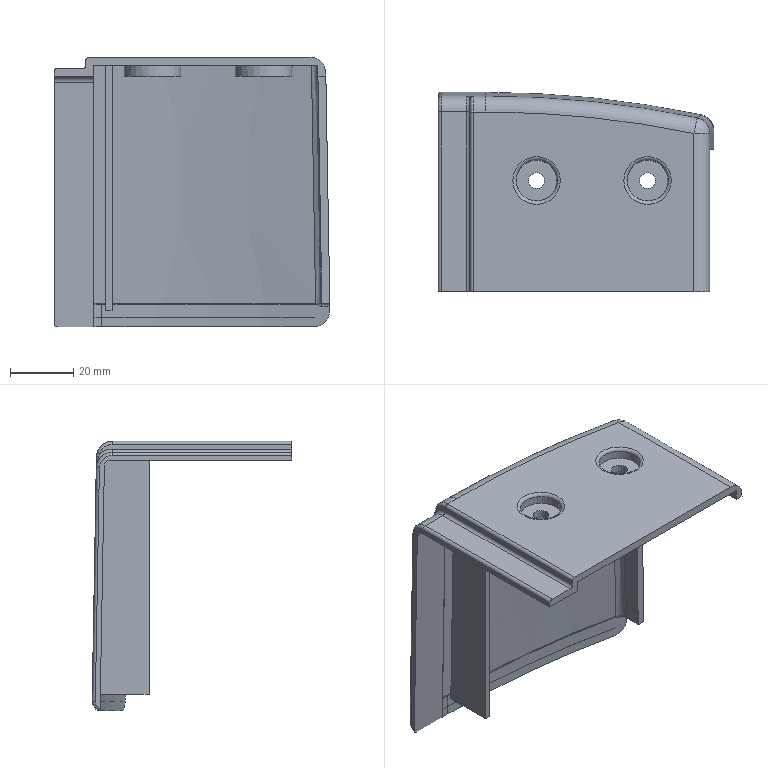Part | STEP file | HGL | 1 solid | 68 faces | box 86.869 x 62.947 x 84.977 mm | volume 34701 mm3 | plane 26 | cylinder 13 | torus 11 | spline 9 | cone 8 | sphere 1 | commonest cylinder face diameters 2 x4 10 x3 5 x2 1 x1 4 x1 6 x1